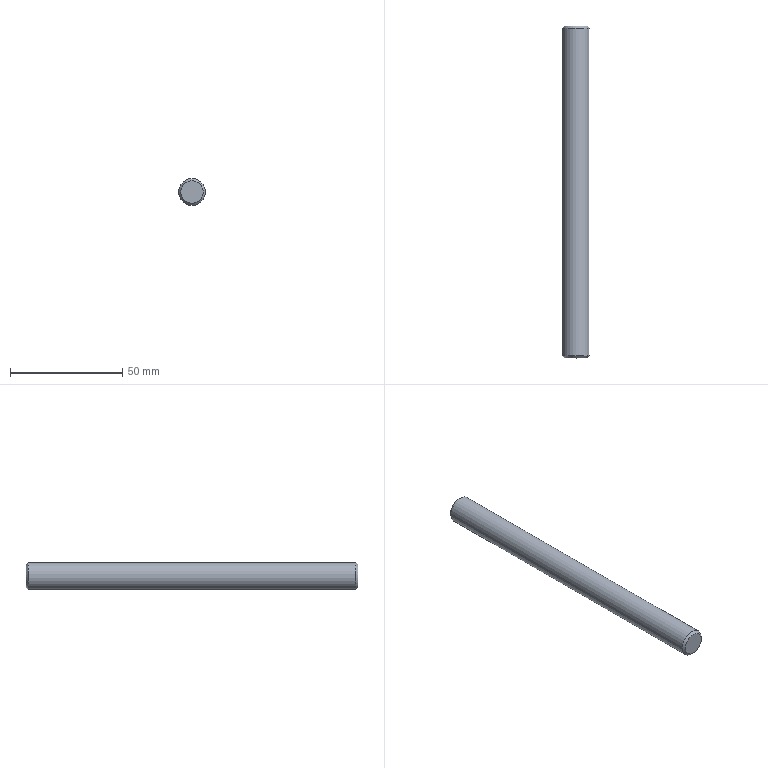Part | NX | features solid 2 | 1 solid | 5 faces | box 12 x 148 x 12 mm | volume 16703 mm3 | plane 2 | cone 2 | cylinder 1 | commonest cylinder face diameters 12 x1
STEP:
#1=CARTESIAN_POINT('',(0.,612.,-123.));
#2=VERTEX_POINT('',#1);
#3=CARTESIAN_POINT('',(0.,612.,-117.));
#4=DIRECTION('',(0.,-1.,0.));
#5=DIRECTION('',(0.,0.,-1.));
#6=AXIS2_PLACEMENT_3D('',#3,#4,#5);
#7=CIRCLE('',#6,6.);
#8=EDGE_CURVE('',#2,#2,#7,.F.);
#9=ORIENTED_EDGE('',*,*,#8,.T.);
#10=EDGE_LOOP('',(#9));
#11=FACE_BOUND('',#10,.T.);
#12=CARTESIAN_POINT('',(0.,758.,-123.));
#13=VERTEX_POINT('',#12);
#14=CARTESIAN_POINT('',(0.,758.,-117.));
#15=DIRECTION('',(0.,-1.,0.));
#16=DIRECTION('',(0.,0.,-1.));
#17=AXIS2_PLACEMENT_3D('',#14,#15,#16);
#18=CIRCLE('',#17,6.);
#19=EDGE_CURVE('',#13,#13,#18,.T.);
#20=ORIENTED_EDGE('',*,*,#19,.T.);
#21=EDGE_LOOP('',(#20));
#22=FACE_BOUND('',#21,.T.);
#23=CARTESIAN_POINT('',(0.,611.,-117.));
#24=DIRECTION('',(0.,1.,0.));
#25=DIRECTION('',(0.,0.,1.));
#26=AXIS2_PLACEMENT_3D('',#23,#24,#25);
#27=CYLINDRICAL_SURFACE('',#26,6.);
#28=ADVANCED_FACE('',(#11,#22),#27,.T.);
#29=CARTESIAN_POINT('',(0.,611.,-122.));
#30=VERTEX_POINT('',#29);
#31=CARTESIAN_POINT('',(0.,611.,-117.));
#32=DIRECTION('',(0.,-1.,0.));
#33=DIRECTION('',(0.,0.,-1.));
#34=AXIS2_PLACEMENT_3D('',#31,#32,#33);
#35=CIRCLE('',#34,5.);
#36=EDGE_CURVE('',#30,#30,#35,.T.);
#37=ORIENTED_EDGE('',*,*,#36,.T.);
#38=EDGE_LOOP('',(#37));
#39=FACE_BOUND('',#38,.T.);
#40=CARTESIAN_POINT('',(0.,611.,-117.));
#41=DIRECTION('',(0.,-1.,0.));
#42=DIRECTION('',(0.,0.,-1.));
#43=AXIS2_PLACEMENT_3D('',#40,#41,#42);
#44=PLANE('',#43);
#45=ADVANCED_FACE('',(#39),#44,.T.);
#46=CARTESIAN_POINT('',(0.,759.,-122.));
#47=VERTEX_POINT('',#46);
#48=CARTESIAN_POINT('',(0.,759.,-117.));
#49=DIRECTION('',(0.,-1.,0.));
#50=DIRECTION('',(0.,0.,-1.));
#51=AXIS2_PLACEMENT_3D('',#48,#49,#50);
#52=CIRCLE('',#51,5.);
#53=EDGE_CURVE('',#47,#47,#52,.F.);
#54=ORIENTED_EDGE('',*,*,#53,.T.);
#55=EDGE_LOOP('',(#54));
#56=FACE_BOUND('',#55,.T.);
#57=CARTESIAN_POINT('',(0.,759.,-117.));
#58=DIRECTION('',(0.,-1.,0.));
#59=DIRECTION('',(0.,0.,-1.));
#60=AXIS2_PLACEMENT_3D('',#57,#58,#59);
#61=PLANE('',#60);
#62=ADVANCED_FACE('',(#56),#61,.F.);
#63=ORIENTED_EDGE('',*,*,#8,.F.);
#64=EDGE_LOOP('',(#63));
#65=FACE_BOUND('',#64,.T.);
#66=ORIENTED_EDGE('',*,*,#36,.F.);
#67=EDGE_LOOP('',(#66));
#68=FACE_BOUND('',#67,.T.);
#69=CARTESIAN_POINT('',(0.,611.,-117.));
#70=DIRECTION('',(0.,1.,0.));
#71=DIRECTION('',(0.,0.,1.));
#72=AXIS2_PLACEMENT_3D('',#69,#70,#71);
#73=CONICAL_SURFACE('',#72,5.,0.7854);
#74=ADVANCED_FACE('',(#65,#68),#73,.T.);
#75=ORIENTED_EDGE('',*,*,#53,.F.);
#76=EDGE_LOOP('',(#75));
#77=FACE_BOUND('',#76,.T.);
#78=ORIENTED_EDGE('',*,*,#19,.F.);
#79=EDGE_LOOP('',(#78));
#80=FACE_BOUND('',#79,.T.);
#81=CARTESIAN_POINT('',(0.,758.,-117.));
#82=DIRECTION('',(0.,-1.,0.));
#83=DIRECTION('',(0.,0.,-1.));
#84=AXIS2_PLACEMENT_3D('',#81,#82,#83);
#85=CONICAL_SURFACE('',#84,6.,0.7854);
#86=ADVANCED_FACE('',(#77,#80),#85,.T.);
#87=CLOSED_SHELL('',(#28,#45,#62,#74,#86));
#88=MANIFOLD_SOLID_BREP('',#87);
#89=(LENGTH_UNIT()NAMED_UNIT(*)SI_UNIT(.MILLI.,.METRE.));
#90=UNCERTAINTY_MEASURE_WITH_UNIT(LENGTH_MEASURE(0.00001),#89,'','');
#91=(NAMED_UNIT(*)PLANE_ANGLE_UNIT()SI_UNIT($,.RADIAN.));
#92=(NAMED_UNIT(*)SI_UNIT($,.STERADIAN.)SOLID_ANGLE_UNIT());
#93=(GEOMETRIC_REPRESENTATION_CONTEXT(3)GLOBAL_UNCERTAINTY_ASSIGNED_CONTEXT((#90))GLOBAL_UNIT_ASSIGNED_CONTEXT((#89,#91,#92))REPRESENTATION_CONTEXT('',''));
#94=ADVANCED_BREP_SHAPE_REPRESENTATION('',(#88),#93);